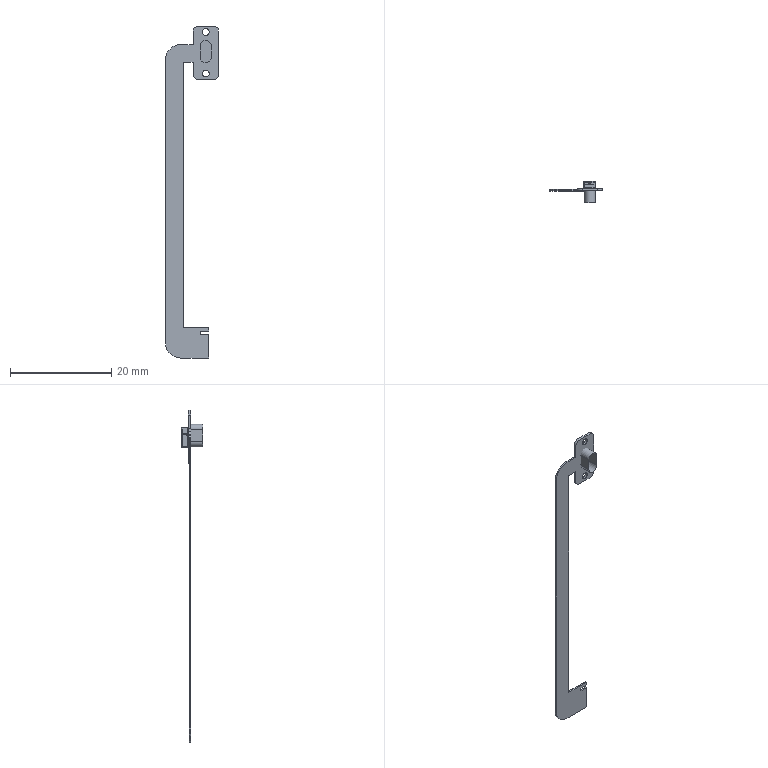Part | Creo | 1 solid | 201 faces | box 10.47 x 4.152 x 65.568 mm | volume 124.944 mm3 | plane 151 | cylinder 46 | sphere 4 | commonest cylinder face diameters 0.01 x12 0.21 x12 0.2 x4 1.3 x4 2 x4 0.8 x2